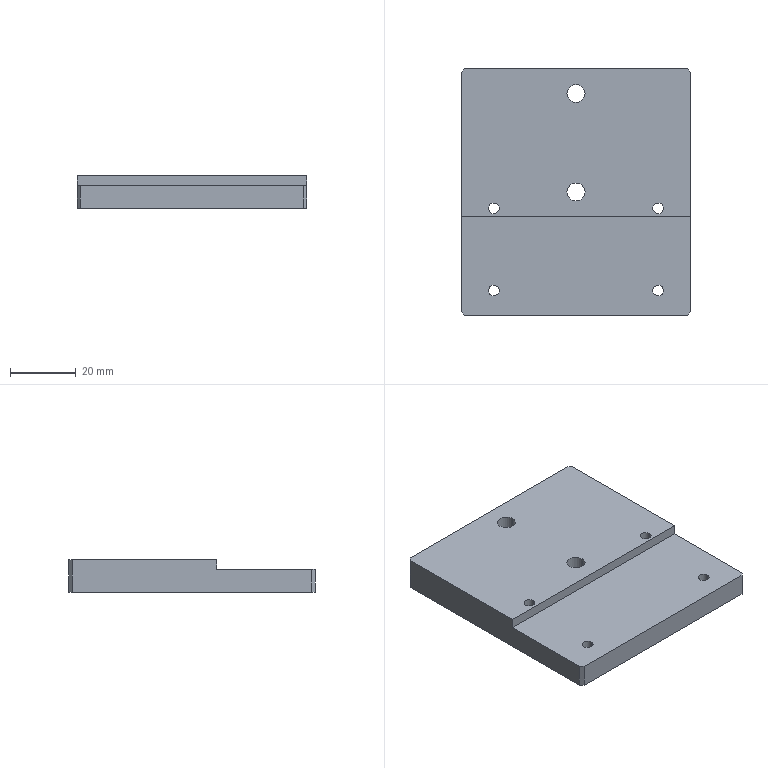Part | SolidWorks | features HoleWzd 2, Chamfer 1, Extrusion 1, ICE 1 | 1 solid | 30 faces | box 70 x 75 x 10 mm | volume 44793 mm3 | cylinder 16 | plane 14 | commonest cylinder face diameters 3.3 x8 5.5 x4 10 x4
STEP:
#1=CARTESIAN_POINT('',(40.,37.5,5.7));
#2=VERTEX_POINT('',#1);
#3=CARTESIAN_POINT('',(30.,37.5,5.7));
#4=VERTEX_POINT('',#3);
#5=CARTESIAN_POINT('',(35.,37.5,5.7));
#6=DIRECTION('',(0.,0.,-1.));
#7=DIRECTION('',(-1.,0.,0.));
#8=AXIS2_PLACEMENT_3D('',#5,#6,#7);
#9=CIRCLE('',#8,5.);
#10=EDGE_CURVE('',#2,#4,#9,.T.);
#11=ORIENTED_EDGE('',*,*,#10,.F.);
#12=CARTESIAN_POINT('',(40.,37.5,0.));
#13=VERTEX_POINT('',#12);
#14=CARTESIAN_POINT('',(40.,37.5,0.));
#15=DIRECTION('',(0.,0.,-1.));
#16=VECTOR('',#15,1000.);
#17=LINE('',#14,#16);
#18=EDGE_CURVE('',#2,#13,#17,.T.);
#19=ORIENTED_EDGE('',*,*,#18,.T.);
#20=CARTESIAN_POINT('',(30.,37.5,0.));
#21=VERTEX_POINT('',#20);
#22=CARTESIAN_POINT('',(35.,37.5,0.));
#23=DIRECTION('',(0.,0.,-1.));
#24=DIRECTION('',(-1.,0.,0.));
#25=AXIS2_PLACEMENT_3D('',#22,#23,#24);
#26=CIRCLE('',#25,5.);
#27=EDGE_CURVE('',#13,#21,#26,.T.);
#28=ORIENTED_EDGE('',*,*,#27,.T.);
#29=CARTESIAN_POINT('',(30.,37.5,0.));
#30=DIRECTION('',(0.,0.,-1.));
#31=VECTOR('',#30,1000.);
#32=LINE('',#29,#31);
#33=EDGE_CURVE('',#4,#21,#32,.T.);
#34=ORIENTED_EDGE('',*,*,#33,.F.);
#35=EDGE_LOOP('',(#11,#19,#28,#34));
#36=FACE_OUTER_BOUND('',#35,.T.);
#37=CARTESIAN_POINT('',(35.,37.5,0.));
#38=DIRECTION('',(0.,0.,-1.));
#39=DIRECTION('',(-1.,0.,0.));
#40=AXIS2_PLACEMENT_3D('',#37,#38,#39);
#41=CYLINDRICAL_SURFACE('',#40,5.);
#42=ADVANCED_FACE('',(#36),#41,.F.);
#43=CARTESIAN_POINT('',(37.75,37.5,10.));
#44=VERTEX_POINT('',#43);
#45=CARTESIAN_POINT('',(32.25,37.5,10.));
#46=VERTEX_POINT('',#45);
#47=CARTESIAN_POINT('',(35.,37.5,10.));
#48=DIRECTION('',(0.,0.,-1.));
#49=DIRECTION('',(-1.,0.,0.));
#50=AXIS2_PLACEMENT_3D('',#47,#48,#49);
#51=CIRCLE('',#50,2.75);
#52=EDGE_CURVE('',#44,#46,#51,.T.);
#53=ORIENTED_EDGE('',*,*,#52,.F.);
#54=CARTESIAN_POINT('',(37.75,37.5,5.7));
#55=VERTEX_POINT('',#54);
#56=CARTESIAN_POINT('',(37.75,37.5,0.));
#57=DIRECTION('',(0.,0.,-1.));
#58=VECTOR('',#57,1000.);
#59=LINE('',#56,#58);
#60=EDGE_CURVE('',#44,#55,#59,.T.);
#61=ORIENTED_EDGE('',*,*,#60,.T.);
#62=CARTESIAN_POINT('',(32.25,37.5,5.7));
#63=VERTEX_POINT('',#62);
#64=CARTESIAN_POINT('',(35.,37.5,5.7));
#65=DIRECTION('',(0.,0.,-1.));
#66=DIRECTION('',(-1.,0.,0.));
#67=AXIS2_PLACEMENT_3D('',#64,#65,#66);
#68=CIRCLE('',#67,2.75);
#69=EDGE_CURVE('',#55,#63,#68,.T.);
#70=ORIENTED_EDGE('',*,*,#69,.T.);
#71=CARTESIAN_POINT('',(32.25,37.5,0.));
#72=DIRECTION('',(0.,0.,-1.));
#73=VECTOR('',#72,1000.);
#74=LINE('',#71,#73);
#75=EDGE_CURVE('',#46,#63,#74,.T.);
#76=ORIENTED_EDGE('',*,*,#75,.F.);
#77=EDGE_LOOP('',(#53,#61,#70,#76));
#78=FACE_OUTER_BOUND('',#77,.T.);
#79=CARTESIAN_POINT('',(35.,37.5,0.));
#80=DIRECTION('',(0.,0.,-1.));
#81=DIRECTION('',(-1.,0.,0.));
#82=AXIS2_PLACEMENT_3D('',#79,#80,#81);
#83=CYLINDRICAL_SURFACE('',#82,2.75);
#84=ADVANCED_FACE('',(#78),#83,.F.);
#85=CARTESIAN_POINT('',(40.,67.5,5.7));
#86=VERTEX_POINT('',#85);
#87=CARTESIAN_POINT('',(30.,67.5,5.7));
#88=VERTEX_POINT('',#87);
#89=CARTESIAN_POINT('',(35.,67.5,5.7));
#90=DIRECTION('',(0.,0.,-1.));
#91=DIRECTION('',(-1.,0.,0.));
#92=AXIS2_PLACEMENT_3D('',#89,#90,#91);
#93=CIRCLE('',#92,5.);
#94=EDGE_CURVE('',#86,#88,#93,.T.);
#95=ORIENTED_EDGE('',*,*,#94,.F.);
#96=CARTESIAN_POINT('',(40.,67.5,0.));
#97=VERTEX_POINT('',#96);
#98=CARTESIAN_POINT('',(40.,67.5,0.));
#99=DIRECTION('',(0.,0.,-1.));
#100=VECTOR('',#99,1000.);
#101=LINE('',#98,#100);
#102=EDGE_CURVE('',#86,#97,#101,.T.);
#103=ORIENTED_EDGE('',*,*,#102,.T.);
#104=CARTESIAN_POINT('',(30.,67.5,0.));
#105=VERTEX_POINT('',#104);
#106=CARTESIAN_POINT('',(35.,67.5,0.));
#107=DIRECTION('',(0.,0.,-1.));
#108=DIRECTION('',(-1.,0.,0.));
#109=AXIS2_PLACEMENT_3D('',#106,#107,#108);
#110=CIRCLE('',#109,5.);
#111=EDGE_CURVE('',#97,#105,#110,.T.);
#112=ORIENTED_EDGE('',*,*,#111,.T.);
#113=CARTESIAN_POINT('',(30.,67.5,0.));
#114=DIRECTION('',(0.,0.,-1.));
#115=VECTOR('',#114,1000.);
#116=LINE('',#113,#115);
#117=EDGE_CURVE('',#88,#105,#116,.T.);
#118=ORIENTED_EDGE('',*,*,#117,.F.);
#119=EDGE_LOOP('',(#95,#103,#112,#118));
#120=FACE_OUTER_BOUND('',#119,.T.);
#121=CARTESIAN_POINT('',(35.,67.5,0.));
#122=DIRECTION('',(0.,0.,-1.));
#123=DIRECTION('',(-1.,0.,0.));
#124=AXIS2_PLACEMENT_3D('',#121,#122,#123);
#125=CYLINDRICAL_SURFACE('',#124,5.);
#126=ADVANCED_FACE('',(#120),#125,.F.);
#127=CARTESIAN_POINT('',(37.75,67.5,10.));
#128=VERTEX_POINT('',#127);
#129=CARTESIAN_POINT('',(32.25,67.5,10.));
#130=VERTEX_POINT('',#129);
#131=CARTESIAN_POINT('',(35.,67.5,10.));
#132=DIRECTION('',(0.,0.,-1.));
#133=DIRECTION('',(-1.,0.,0.));
#134=AXIS2_PLACEMENT_3D('',#131,#132,#133);
#135=CIRCLE('',#134,2.75);
#136=EDGE_CURVE('',#128,#130,#135,.T.);
#137=ORIENTED_EDGE('',*,*,#136,.F.);
#138=CARTESIAN_POINT('',(37.75,67.5,5.7));
#139=VERTEX_POINT('',#138);
#140=CARTESIAN_POINT('',(37.75,67.5,0.));
#141=DIRECTION('',(0.,0.,-1.));
#142=VECTOR('',#141,1000.);
#143=LINE('',#140,#142);
#144=EDGE_CURVE('',#128,#139,#143,.T.);
#145=ORIENTED_EDGE('',*,*,#144,.T.);
#146=CARTESIAN_POINT('',(32.25,67.5,5.7));
#147=VERTEX_POINT('',#146);
#148=CARTESIAN_POINT('',(35.,67.5,5.7));
#149=DIRECTION('',(0.,0.,-1.));
#150=DIRECTION('',(-1.,0.,0.));
#151=AXIS2_PLACEMENT_3D('',#148,#149,#150);
#152=CIRCLE('',#151,2.75);
#153=EDGE_CURVE('',#139,#147,#152,.T.);
#154=ORIENTED_EDGE('',*,*,#153,.T.);
#155=CARTESIAN_POINT('',(32.25,67.5,0.));
#156=DIRECTION('',(0.,0.,-1.));
#157=VECTOR('',#156,1000.);
#158=LINE('',#155,#157);
#159=EDGE_CURVE('',#130,#147,#158,.T.);
#160=ORIENTED_EDGE('',*,*,#159,.F.);
#161=EDGE_LOOP('',(#137,#145,#154,#160));
#162=FACE_OUTER_BOUND('',#161,.T.);
#163=CARTESIAN_POINT('',(35.,67.5,0.));
#164=DIRECTION('',(0.,0.,-1.));
#165=DIRECTION('',(-1.,0.,0.));
#166=AXIS2_PLACEMENT_3D('',#163,#164,#165);
#167=CYLINDRICAL_SURFACE('',#166,2.75);
#168=ADVANCED_FACE('',(#162),#167,.F.);
#169=CARTESIAN_POINT('',(11.65,7.5,7.));
#170=VERTEX_POINT('',#169);
#171=CARTESIAN_POINT('',(8.35,7.5,7.));
#172=VERTEX_POINT('',#171);
#173=CARTESIAN_POINT('',(10.,7.5,7.));
#174=DIRECTION('',(0.,0.,-1.));
#175=DIRECTION('',(-1.,0.,0.));
#176=AXIS2_PLACEMENT_3D('',#173,#174,#175);
#177=CIRCLE('',#176,1.65);
#178=EDGE_CURVE('',#170,#172,#177,.T.);
#179=ORIENTED_EDGE('',*,*,#178,.F.);
#180=CARTESIAN_POINT('',(11.65,7.5,0.));
#181=VERTEX_POINT('',#180);
#182=CARTESIAN_POINT('',(11.65,7.5,0.));
#183=DIRECTION('',(0.,0.,-1.));
#184=VECTOR('',#183,1000.);
#185=LINE('',#182,#184);
#186=EDGE_CURVE('',#170,#181,#185,.T.);
#187=ORIENTED_EDGE('',*,*,#186,.T.);
#188=CARTESIAN_POINT('',(8.35,7.5,0.));
#189=VERTEX_POINT('',#188);
#190=CARTESIAN_POINT('',(10.,7.5,0.));
#191=DIRECTION('',(0.,0.,-1.));
#192=DIRECTION('',(-1.,0.,0.));
#193=AXIS2_PLACEMENT_3D('',#190,#191,#192);
#194=CIRCLE('',#193,1.65);
#195=EDGE_CURVE('',#181,#189,#194,.T.);
#196=ORIENTED_EDGE('',*,*,#195,.T.);
#197=CARTESIAN_POINT('',(8.35,7.5,0.));
#198=DIRECTION('',(0.,0.,-1.));
#199=VECTOR('',#198,1000.);
#200=LINE('',#197,#199);
#201=EDGE_CURVE('',#172,#189,#200,.T.);
#202=ORIENTED_EDGE('',*,*,#201,.F.);
#203=EDGE_LOOP('',(#179,#187,#196,#202));
#204=FACE_OUTER_BOUND('',#203,.T.);
#205=CARTESIAN_POINT('',(10.,7.5,0.));
#206=DIRECTION('',(0.,0.,-1.));
#207=DIRECTION('',(-1.,0.,0.));
#208=AXIS2_PLACEMENT_3D('',#205,#206,#207);
#209=CYLINDRICAL_SURFACE('',#208,1.65);
#210=ADVANCED_FACE('',(#204),#209,.F.);
#211=CARTESIAN_POINT('',(11.65,32.5,10.));
#212=VERTEX_POINT('',#211);
#213=CARTESIAN_POINT('',(8.35,32.5,10.));
#214=VERTEX_POINT('',#213);
#215=CARTESIAN_POINT('',(10.,32.5,10.));
#216=DIRECTION('',(0.,0.,-1.));
#217=DIRECTION('',(-1.,0.,0.));
#218=AXIS2_PLACEMENT_3D('',#215,#216,#217);
#219=CIRCLE('',#218,1.65);
#220=EDGE_CURVE('',#212,#214,#219,.T.);
#221=ORIENTED_EDGE('',*,*,#220,.F.);
#222=CARTESIAN_POINT('',(11.65,32.5,0.));
#223=VERTEX_POINT('',#222);
#224=CARTESIAN_POINT('',(11.65,32.5,0.));
#225=DIRECTION('',(0.,0.,-1.));
#226=VECTOR('',#225,1000.);
#227=LINE('',#224,#226);
#228=EDGE_CURVE('',#212,#223,#227,.T.);
#229=ORIENTED_EDGE('',*,*,#228,.T.);
#230=CARTESIAN_POINT('',(8.35,32.5,0.));
#231=VERTEX_POINT('',#230);
#232=CARTESIAN_POINT('',(10.,32.5,0.));
#233=DIRECTION('',(0.,0.,-1.));
#234=DIRECTION('',(-1.,0.,0.));
#235=AXIS2_PLACEMENT_3D('',#232,#233,#234);
#236=CIRCLE('',#235,1.65);
#237=EDGE_CURVE('',#223,#231,#236,.T.);
#238=ORIENTED_EDGE('',*,*,#237,.T.);
#239=CARTESIAN_POINT('',(8.35,32.5,0.));
#240=DIRECTION('',(0.,0.,-1.));
#241=VECTOR('',#240,1000.);
#242=LINE('',#239,#241);
#243=EDGE_CURVE('',#214,#231,#242,.T.);
#244=ORIENTED_EDGE('',*,*,#243,.F.);
#245=EDGE_LOOP('',(#221,#229,#238,#244));
#246=FACE_OUTER_BOUND('',#245,.T.);
#247=CARTESIAN_POINT('',(10.,32.5,0.));
#248=DIRECTION('',(0.,0.,-1.));
#249=DIRECTION('',(-1.,0.,0.));
#250=AXIS2_PLACEMENT_3D('',#247,#248,#249);
#251=CYLINDRICAL_SURFACE('',#250,1.65);
#252=ADVANCED_FACE('',(#246),#251,.F.);
#253=CARTESIAN_POINT('',(61.65,7.5,7.));
#254=VERTEX_POINT('',#253);
#255=CARTESIAN_POINT('',(58.35,7.5,7.));
#256=VERTEX_POINT('',#255);
#257=CARTESIAN_POINT('',(60.,7.5,7.));
#258=DIRECTION('',(0.,0.,-1.));
#259=DIRECTION('',(-1.,0.,0.));
#260=AXIS2_PLACEMENT_3D('',#257,#258,#259);
#261=CIRCLE('',#260,1.65);
#262=EDGE_CURVE('',#254,#256,#261,.T.);
#263=ORIENTED_EDGE('',*,*,#262,.F.);
#264=CARTESIAN_POINT('',(61.65,7.5,0.));
#265=VERTEX_POINT('',#264);
#266=CARTESIAN_POINT('',(61.65,7.5,0.));
#267=DIRECTION('',(0.,0.,-1.));
#268=VECTOR('',#267,1000.);
#269=LINE('',#266,#268);
#270=EDGE_CURVE('',#254,#265,#269,.T.);
#271=ORIENTED_EDGE('',*,*,#270,.T.);
#272=CARTESIAN_POINT('',(58.35,7.5,0.));
#273=VERTEX_POINT('',#272);
#274=CARTESIAN_POINT('',(60.,7.5,0.));
#275=DIRECTION('',(0.,0.,-1.));
#276=DIRECTION('',(-1.,0.,0.));
#277=AXIS2_PLACEMENT_3D('',#274,#275,#276);
#278=CIRCLE('',#277,1.65);
#279=EDGE_CURVE('',#265,#273,#278,.T.);
#280=ORIENTED_EDGE('',*,*,#279,.T.);
#281=CARTESIAN_POINT('',(58.35,7.5,0.));
#282=DIRECTION('',(0.,0.,-1.));
#283=VECTOR('',#282,1000.);
#284=LINE('',#281,#283);
#285=EDGE_CURVE('',#256,#273,#284,.T.);
#286=ORIENTED_EDGE('',*,*,#285,.F.);
#287=EDGE_LOOP('',(#263,#271,#280,#286));
#288=FACE_OUTER_BOUND('',#287,.T.);
#289=CARTESIAN_POINT('',(60.,7.5,0.));
#290=DIRECTION('',(0.,0.,-1.));
#291=DIRECTION('',(-1.,0.,0.));
#292=AXIS2_PLACEMENT_3D('',#289,#290,#291);
#293=CYLINDRICAL_SURFACE('',#292,1.65);
#294=ADVANCED_FACE('',(#288),#293,.F.);
#295=CARTESIAN_POINT('',(61.65,32.5,10.));
#296=VERTEX_POINT('',#295);
#297=CARTESIAN_POINT('',(58.35,32.5,10.));
#298=VERTEX_POINT('',#297);
#299=CARTESIAN_POINT('',(60.,32.5,10.));
#300=DIRECTION('',(0.,0.,-1.));
#301=DIRECTION('',(-1.,0.,0.));
#302=AXIS2_PLACEMENT_3D('',#299,#300,#301);
#303=CIRCLE('',#302,1.65);
#304=EDGE_CURVE('',#296,#298,#303,.T.);
#305=ORIENTED_EDGE('',*,*,#304,.F.);
#306=CARTESIAN_POINT('',(61.65,32.5,0.));
#307=VERTEX_POINT('',#306);
#308=CARTESIAN_POINT('',(61.65,32.5,0.));
#309=DIRECTION('',(0.,0.,-1.));
#310=VECTOR('',#309,1000.);
#311=LINE('',#308,#310);
#312=EDGE_CURVE('',#296,#307,#311,.T.);
#313=ORIENTED_EDGE('',*,*,#312,.T.);
#314=CARTESIAN_POINT('',(58.35,32.5,0.));
#315=VERTEX_POINT('',#314);
#316=CARTESIAN_POINT('',(60.,32.5,0.));
#317=DIRECTION('',(0.,0.,-1.));
#318=DIRECTION('',(-1.,0.,0.));
#319=AXIS2_PLACEMENT_3D('',#316,#317,#318);
#320=CIRCLE('',#319,1.65);
#321=EDGE_CURVE('',#307,#315,#320,.T.);
#322=ORIENTED_EDGE('',*,*,#321,.T.);
#323=CARTESIAN_POINT('',(58.35,32.5,0.));
#324=DIRECTION('',(0.,0.,-1.));
#325=VECTOR('',#324,1000.);
#326=LINE('',#323,#325);
#327=EDGE_CURVE('',#298,#315,#326,.T.);
#328=ORIENTED_EDGE('',*,*,#327,.F.);
#329=EDGE_LOOP('',(#305,#313,#322,#328));
#330=FACE_OUTER_BOUND('',#329,.T.);
#331=CARTESIAN_POINT('',(60.,32.5,0.));
#332=DIRECTION('',(0.,0.,-1.));
#333=DIRECTION('',(-1.,0.,0.));
#334=AXIS2_PLACEMENT_3D('',#331,#332,#333);
#335=CYLINDRICAL_SURFACE('',#334,1.65);
#336=ADVANCED_FACE('',(#330),#335,.F.);
#337=CARTESIAN_POINT('',(0.,74.,0.));
#338=VERTEX_POINT('',#337);
#339=CARTESIAN_POINT('',(0.,1.,0.));
#340=VERTEX_POINT('',#339);
#341=CARTESIAN_POINT('',(0.,0.,0.));
#342=DIRECTION('',(0.,-1.,0.));
#343=VECTOR('',#342,1000.);
#344=LINE('',#341,#343);
#345=EDGE_CURVE('',#338,#340,#344,.T.);
#346=ORIENTED_EDGE('',*,*,#345,.T.);
#347=CARTESIAN_POINT('',(0.,1.,7.));
#348=VERTEX_POINT('',#347);
#349=CARTESIAN_POINT('',(0.,1.,10.));
#350=DIRECTION('',(0.,0.,1.));
#351=VECTOR('',#350,1000.);
#352=LINE('',#349,#351);
#353=EDGE_CURVE('',#340,#348,#352,.T.);
#354=ORIENTED_EDGE('',*,*,#353,.T.);
#355=CARTESIAN_POINT('',(0.,30.,7.));
#356=VERTEX_POINT('',#355);
#357=CARTESIAN_POINT('',(0.,0.,7.));
#358=DIRECTION('',(0.,-1.,0.));
#359=VECTOR('',#358,1000.);
#360=LINE('',#357,#359);
#361=EDGE_CURVE('',#356,#348,#360,.T.);
#362=ORIENTED_EDGE('',*,*,#361,.F.);
#363=CARTESIAN_POINT('',(0.,30.,10.));
#364=VERTEX_POINT('',#363);
#365=CARTESIAN_POINT('',(0.,30.,10.));
#366=DIRECTION('',(0.,0.,-1.));
#367=VECTOR('',#366,1000.);
#368=LINE('',#365,#367);
#369=EDGE_CURVE('',#364,#356,#368,.T.);
#370=ORIENTED_EDGE('',*,*,#369,.F.);
#371=CARTESIAN_POINT('',(0.,74.,10.));
#372=VERTEX_POINT('',#371);
#373=CARTESIAN_POINT('',(0.,0.,10.));
#374=DIRECTION('',(0.,-1.,0.));
#375=VECTOR('',#374,1000.);
#376=LINE('',#373,#375);
#377=EDGE_CURVE('',#372,#364,#376,.T.);
#378=ORIENTED_EDGE('',*,*,#377,.F.);
#379=CARTESIAN_POINT('',(0.,74.,10.));
#380=DIRECTION('',(0.,0.,-1.));
#381=VECTOR('',#380,1000.);
#382=LINE('',#379,#381);
#383=EDGE_CURVE('',#372,#338,#382,.T.);
#384=ORIENTED_EDGE('',*,*,#383,.T.);
#385=EDGE_LOOP('',(#346,#354,#362,#370,#378,#384));
#386=FACE_OUTER_BOUND('',#385,.T.);
#387=CARTESIAN_POINT('',(0.,0.,10.));
#388=DIRECTION('',(1.,0.,0.));
#389=DIRECTION('',(0.,0.,-1.));
#390=AXIS2_PLACEMENT_3D('',#387,#388,#389);
#391=PLANE('',#390);
#392=ADVANCED_FACE('',(#386),#391,.F.);
#393=CARTESIAN_POINT('',(1.,0.,0.));
#394=VERTEX_POINT('',#393);
#395=CARTESIAN_POINT('',(69.,0.,0.));
#396=VERTEX_POINT('',#395);
#397=CARTESIAN_POINT('',(0.,0.,0.));
#398=DIRECTION('',(1.,0.,0.));
#399=VECTOR('',#398,1000.);
#400=LINE('',#397,#399);
#401=EDGE_CURVE('',#394,#396,#400,.T.);
#402=ORIENTED_EDGE('',*,*,#401,.T.);
#403=CARTESIAN_POINT('',(69.,0.,7.));
#404=VERTEX_POINT('',#403);
#405=CARTESIAN_POINT('',(69.,0.,10.));
#406=DIRECTION('',(0.,0.,1.));
#407=VECTOR('',#406,1000.);
#408=LINE('',#405,#407);
#409=EDGE_CURVE('',#396,#404,#408,.T.);
#410=ORIENTED_EDGE('',*,*,#409,.T.);
#411=CARTESIAN_POINT('',(1.,0.,7.));
#412=VERTEX_POINT('',#411);
#413=CARTESIAN_POINT('',(70.,0.,7.));
#414=DIRECTION('',(-1.,0.,0.));
#415=VECTOR('',#414,1000.);
#416=LINE('',#413,#415);
#417=EDGE_CURVE('',#404,#412,#416,.T.);
#418=ORIENTED_EDGE('',*,*,#417,.T.);
#419=CARTESIAN_POINT('',(1.,0.,10.));
#420=DIRECTION('',(0.,0.,-1.));
#421=VECTOR('',#420,1000.);
#422=LINE('',#419,#421);
#423=EDGE_CURVE('',#412,#394,#422,.T.);
#424=ORIENTED_EDGE('',*,*,#423,.T.);
#425=EDGE_LOOP('',(#402,#410,#418,#424));
#426=FACE_OUTER_BOUND('',#425,.T.);
#427=CARTESIAN_POINT('',(0.,0.,10.));
#428=DIRECTION('',(0.,1.,0.));
#429=DIRECTION('',(0.,0.,1.));
#430=AXIS2_PLACEMENT_3D('',#427,#428,#429);
#431=PLANE('',#430);
#432=ADVANCED_FACE('',(#426),#431,.F.);
#433=CARTESIAN_POINT('',(70.,30.,7.));
#434=VERTEX_POINT('',#433);
#435=CARTESIAN_POINT('',(70.,1.,7.));
#436=VERTEX_POINT('',#435);
#437=CARTESIAN_POINT('',(70.,0.,7.));
#438=DIRECTION('',(0.,-1.,0.));
#439=VECTOR('',#438,1000.);
#440=LINE('',#437,#439);
#441=EDGE_CURVE('',#434,#436,#440,.T.);
#442=ORIENTED_EDGE('',*,*,#441,.T.);
#443=CARTESIAN_POINT('',(70.,1.,0.));
#444=VERTEX_POINT('',#443);
#445=CARTESIAN_POINT('',(70.,1.,10.));
#446=DIRECTION('',(0.,0.,-1.));
#447=VECTOR('',#446,1000.);
#448=LINE('',#445,#447);
#449=EDGE_CURVE('',#436,#444,#448,.T.);
#450=ORIENTED_EDGE('',*,*,#449,.T.);
#451=CARTESIAN_POINT('',(70.,74.,0.));
#452=VERTEX_POINT('',#451);
#453=CARTESIAN_POINT('',(70.,0.,0.));
#454=DIRECTION('',(0.,1.,0.));
#455=VECTOR('',#454,1000.);
#456=LINE('',#453,#455);
#457=EDGE_CURVE('',#444,#452,#456,.T.);
#458=ORIENTED_EDGE('',*,*,#457,.T.);
#459=CARTESIAN_POINT('',(70.,74.,10.));
#460=VERTEX_POINT('',#459);
#461=CARTESIAN_POINT('',(70.,74.,10.));
#462=DIRECTION('',(0.,0.,1.));
#463=VECTOR('',#462,1000.);
#464=LINE('',#461,#463);
#465=EDGE_CURVE('',#452,#460,#464,.T.);
#466=ORIENTED_EDGE('',*,*,#465,.T.);
#467=CARTESIAN_POINT('',(70.,30.,10.));
#468=VERTEX_POINT('',#467);
#469=CARTESIAN_POINT('',(70.,0.,10.));
#470=DIRECTION('',(0.,1.,0.));
#471=VECTOR('',#470,1000.);
#472=LINE('',#469,#471);
#473=EDGE_CURVE('',#468,#460,#472,.T.);
#474=ORIENTED_EDGE('',*,*,#473,.F.);
#475=CARTESIAN_POINT('',(70.,30.,10.));
#476=DIRECTION('',(0.,0.,-1.));
#477=VECTOR('',#476,1000.);
#478=LINE('',#475,#477);
#479=EDGE_CURVE('',#468,#434,#478,.T.);
#480=ORIENTED_EDGE('',*,*,#479,.T.);
#481=EDGE_LOOP('',(#442,#450,#458,#466,#474,#480));
#482=FACE_OUTER_BOUND('',#481,.T.);
#483=CARTESIAN_POINT('',(70.,0.,10.));
#484=DIRECTION('',(-1.,0.,0.));
#485=DIRECTION('',(0.,0.,1.));
#486=AXIS2_PLACEMENT_3D('',#483,#484,#485);
#487=PLANE('',#486);
#488=ADVANCED_FACE('',(#482),#487,.F.);
#489=CARTESIAN_POINT('',(69.,75.,0.));
#490=VERTEX_POINT('',#489);
#491=CARTESIAN_POINT('',(1.,75.,0.));
#492=VERTEX_POINT('',#491);
#493=CARTESIAN_POINT('',(0.,75.,0.));
#494=DIRECTION('',(-1.,0.,0.));
#495=VECTOR('',#494,1000.);
#496=LINE('',#493,#495);
#497=EDGE_CURVE('',#490,#492,#496,.T.);
#498=ORIENTED_EDGE('',*,*,#497,.T.);
#499=CARTESIAN_POINT('',(1.,75.,10.));
#500=VERTEX_POINT('',#499);
#501=CARTESIAN_POINT('',(1.,75.,10.));
#502=DIRECTION('',(0.,0.,1.));
#503=VECTOR('',#502,1000.);
#504=LINE('',#501,#503);
#505=EDGE_CURVE('',#492,#500,#504,.T.);
#506=ORIENTED_EDGE('',*,*,#505,.T.);
#507=CARTESIAN_POINT('',(69.,75.,10.));
#508=VERTEX_POINT('',#507);
#509=CARTESIAN_POINT('',(0.,75.,10.));
#510=DIRECTION('',(-1.,0.,0.));
#511=VECTOR('',#510,1000.);
#512=LINE('',#509,#511);
#513=EDGE_CURVE('',#508,#500,#512,.T.);
#514=ORIENTED_EDGE('',*,*,#513,.F.);
#515=CARTESIAN_POINT('',(69.,75.,10.));
#516=DIRECTION('',(0.,0.,-1.));
#517=VECTOR('',#516,1000.);
#518=LINE('',#515,#517);
#519=EDGE_CURVE('',#508,#490,#518,.T.);
#520=ORIENTED_EDGE('',*,*,#519,.T.);
#521=EDGE_LOOP('',(#498,#506,#514,#520));
#522=FACE_OUTER_BOUND('',#521,.T.);
#523=CARTESIAN_POINT('',(0.,75.,10.));
#524=DIRECTION('',(0.,-1.,0.));
#525=DIRECTION('',(0.,0.,-1.));
#526=AXIS2_PLACEMENT_3D('',#523,#524,#525);
#527=PLANE('',#526);
#528=ADVANCED_FACE('',(#522),#527,.F.);
#529=CARTESIAN_POINT('',(35.,37.5,10.));
#530=DIRECTION('',(0.,0.,-1.));
#531=DIRECTION('',(-1.,0.,0.));
#532=AXIS2_PLACEMENT_3D('',#529,#530,#531);
#533=CIRCLE('',#532,2.75);
#534=EDGE_CURVE('',#46,#44,#533,.T.);
#535=ORIENTED_EDGE('',*,*,#534,.T.);
#536=ORIENTED_EDGE('',*,*,#52,.T.);
#537=EDGE_LOOP('',(#535,#536));
#538=FACE_BOUND('',#537,.T.);
#539=CARTESIAN_POINT('',(35.,67.5,10.));
#540=DIRECTION('',(0.,0.,-1.));
#541=DIRECTION('',(-1.,0.,0.));
#542=AXIS2_PLACEMENT_3D('',#539,#540,#541);
#543=CIRCLE('',#542,2.75);
#544=EDGE_CURVE('',#130,#128,#543,.T.);
#545=ORIENTED_EDGE('',*,*,#544,.T.);
#546=ORIENTED_EDGE('',*,*,#136,.T.);
#547=EDGE_LOOP('',(#545,#546));
#548=FACE_BOUND('',#547,.T.);
#549=CARTESIAN_POINT('',(10.,32.5,10.));
#550=DIRECTION('',(0.,0.,-1.));
#551=DIRECTION('',(-1.,0.,0.));
#552=AXIS2_PLACEMENT_3D('',#549,#550,#551);
#553=CIRCLE('',#552,1.65);
#554=EDGE_CURVE('',#214,#212,#553,.T.);
#555=ORIENTED_EDGE('',*,*,#554,.T.);
#556=ORIENTED_EDGE('',*,*,#220,.T.);
#557=EDGE_LOOP('',(#555,#556));
#558=FACE_BOUND('',#557,.T.);
#559=CARTESIAN_POINT('',(60.,32.5,10.));
#560=DIRECTION('',(0.,0.,-1.));
#561=DIRECTION('',(-1.,0.,0.));
#562=AXIS2_PLACEMENT_3D('',#559,#560,#561);
#563=CIRCLE('',#562,1.65);
#564=EDGE_CURVE('',#298,#296,#563,.T.);
#565=ORIENTED_EDGE('',*,*,#564,.T.);
#566=ORIENTED_EDGE('',*,*,#304,.T.);
#567=EDGE_LOOP('',(#565,#566));
#568=FACE_BOUND('',#567,.T.);
#569=ORIENTED_EDGE('',*,*,#513,.T.);
#570=CARTESIAN_POINT('',(0.,74.,10.));
#571=DIRECTION('',(-0.7071,-0.7071,0.));
#572=VECTOR('',#571,1000.);
#573=LINE('',#570,#572);
#574=EDGE_CURVE('',#500,#372,#573,.T.);
#575=ORIENTED_EDGE('',*,*,#574,.T.);
#576=ORIENTED_EDGE('',*,*,#377,.T.);
#577=CARTESIAN_POINT('',(70.,30.,10.));
#578=DIRECTION('',(-1.,0.,0.));
#579=VECTOR('',#578,1000.);
#580=LINE('',#577,#579);
#581=EDGE_CURVE('',#468,#364,#580,.T.);
#582=ORIENTED_EDGE('',*,*,#581,.F.);
#583=ORIENTED_EDGE('',*,*,#473,.T.);
#584=CARTESIAN_POINT('',(69.,75.,10.));
#585=DIRECTION('',(-0.7071,0.7071,0.));
#586=VECTOR('',#585,1000.);
#587=LINE('',#584,#586);
#588=EDGE_CURVE('',#460,#508,#587,.T.);
#589=ORIENTED_EDGE('',*,*,#588,.T.);
#590=EDGE_LOOP('',(#569,#575,#576,#582,#583,#589));
#591=FACE_OUTER_BOUND('',#590,.T.);
#592=CARTESIAN_POINT('',(0.,75.,10.));
#593=DIRECTION('',(0.,0.,-1.));
#594=DIRECTION('',(-1.,0.,0.));
#595=AXIS2_PLACEMENT_3D('',#592,#593,#594);
#596=PLANE('',#595);
#597=ADVANCED_FACE('',(#538,#548,#558,#568,#591),#596,.F.);
#598=CARTESIAN_POINT('',(35.,37.5,0.));
#599=DIRECTION('',(0.,0.,-1.));
#600=DIRECTION('',(-1.,0.,0.));
#601=AXIS2_PLACEMENT_3D('',#598,#599,#600);
#602=CIRCLE('',#601,5.);
#603=EDGE_CURVE('',#21,#13,#602,.T.);
#604=ORIENTED_EDGE('',*,*,#603,.F.);
#605=ORIENTED_EDGE('',*,*,#27,.F.);
#606=EDGE_LOOP('',(#604,#605));
#607=FACE_BOUND('',#606,.T.);
#608=CARTESIAN_POINT('',(35.,67.5,0.));
#609=DIRECTION('',(0.,0.,-1.));
#610=DIRECTION('',(-1.,0.,0.));
#611=AXIS2_PLACEMENT_3D('',#608,#609,#610);
#612=CIRCLE('',#611,5.);
#613=EDGE_CURVE('',#105,#97,#612,.T.);
#614=ORIENTED_EDGE('',*,*,#613,.F.);
#615=ORIENTED_EDGE('',*,*,#111,.F.);
#616=EDGE_LOOP('',(#614,#615));
#617=FACE_BOUND('',#616,.T.);
#618=CARTESIAN_POINT('',(10.,7.5,0.));
#619=DIRECTION('',(0.,0.,-1.));
#620=DIRECTION('',(-1.,0.,0.));
#621=AXIS2_PLACEMENT_3D('',#618,#619,#620);
#622=CIRCLE('',#621,1.65);
#623=EDGE_CURVE('',#189,#181,#622,.T.);
#624=ORIENTED_EDGE('',*,*,#623,.F.);
#625=ORIENTED_EDGE('',*,*,#195,.F.);
#626=EDGE_LOOP('',(#624,#625));
#627=FACE_BOUND('',#626,.T.);
#628=CARTESIAN_POINT('',(10.,32.5,0.));
#629=DIRECTION('',(0.,0.,-1.));
#630=DIRECTION('',(-1.,0.,0.));
#631=AXIS2_PLACEMENT_3D('',#628,#629,#630);
#632=CIRCLE('',#631,1.65);
#633=EDGE_CURVE('',#231,#223,#632,.T.);
#634=ORIENTED_EDGE('',*,*,#633,.F.);
#635=ORIENTED_EDGE('',*,*,#237,.F.);
#636=EDGE_LOOP('',(#634,#635));
#637=FACE_BOUND('',#636,.T.);
#638=CARTESIAN_POINT('',(60.,7.5,0.));
#639=DIRECTION('',(0.,0.,-1.));
#640=DIRECTION('',(-1.,0.,0.));
#641=AXIS2_PLACEMENT_3D('',#638,#639,#640);
#642=CIRCLE('',#641,1.65);
#643=EDGE_CURVE('',#273,#265,#642,.T.);
#644=ORIENTED_EDGE('',*,*,#643,.F.);
#645=ORIENTED_EDGE('',*,*,#279,.F.);
#646=EDGE_LOOP('',(#644,#645));
#647=FACE_BOUND('',#646,.T.);
#648=CARTESIAN_POINT('',(60.,32.5,0.));
#649=DIRECTION('',(0.,0.,-1.));
#650=DIRECTION('',(-1.,0.,0.));
#651=AXIS2_PLACEMENT_3D('',#648,#649,#650);
#652=CIRCLE('',#651,1.65);
#653=EDGE_CURVE('',#315,#307,#652,.T.);
#654=ORIENTED_EDGE('',*,*,#653,.F.);
#655=ORIENTED_EDGE('',*,*,#321,.F.);
#656=EDGE_LOOP('',(#654,#655));
#657=FACE_BOUND('',#656,.T.);
#658=ORIENTED_EDGE('',*,*,#457,.F.);
#659=CARTESIAN_POINT('',(72.,3.,0.));
#660=DIRECTION('',(-0.7071,-0.7071,0.));
#661=VECTOR('',#660,1000.);
#662=LINE('',#659,#661);
#663=EDGE_CURVE('',#444,#396,#662,.T.);
#664=ORIENTED_EDGE('',*,*,#663,.T.);
#665=ORIENTED_EDGE('',*,*,#401,.F.);
#666=CARTESIAN_POINT('',(-37.,38.,0.));
#667=DIRECTION('',(-0.7071,0.7071,0.));
#668=VECTOR('',#667,1000.);
#669=LINE('',#666,#668);
#670=EDGE_CURVE('',#394,#340,#669,.T.);
#671=ORIENTED_EDGE('',*,*,#670,.T.);
#672=ORIENTED_EDGE('',*,*,#345,.F.);
#673=CARTESIAN_POINT('',(0.5,74.5,0.));
#674=DIRECTION('',(0.7071,0.7071,0.));
#675=VECTOR('',#674,1000.);
#676=LINE('',#673,#675);
#677=EDGE_CURVE('',#338,#492,#676,.T.);
#678=ORIENTED_EDGE('',*,*,#677,.T.);
#679=ORIENTED_EDGE('',*,*,#497,.F.);
#680=CARTESIAN_POINT('',(34.5,109.5,0.));
#681=DIRECTION('',(0.7071,-0.7071,0.));
#682=VECTOR('',#681,1000.);
#683=LINE('',#680,#682);
#684=EDGE_CURVE('',#490,#452,#683,.T.);
#685=ORIENTED_EDGE('',*,*,#684,.T.);
#686=EDGE_LOOP('',(#658,#664,#665,#671,#672,#678,#679,#685));
#687=FACE_OUTER_BOUND('',#686,.T.);
#688=CARTESIAN_POINT('',(0.,75.,0.));
#689=DIRECTION('',(0.,0.,-1.));
#690=DIRECTION('',(-1.,0.,0.));
#691=AXIS2_PLACEMENT_3D('',#688,#689,#690);
#692=PLANE('',#691);
#693=ADVANCED_FACE('',(#607,#617,#627,#637,#647,#657,#687),#692,.T.);
#694=CARTESIAN_POINT('',(10.,7.5,7.));
#695=DIRECTION('',(0.,0.,-1.));
#696=DIRECTION('',(-1.,0.,0.));
#697=AXIS2_PLACEMENT_3D('',#694,#695,#696);
#698=CIRCLE('',#697,1.65);
#699=EDGE_CURVE('',#172,#170,#698,.T.);
#700=ORIENTED_EDGE('',*,*,#699,.T.);
#701=ORIENTED_EDGE('',*,*,#178,.T.);
#702=EDGE_LOOP('',(#700,#701));
#703=FACE_BOUND('',#702,.T.);
#704=CARTESIAN_POINT('',(60.,7.5,7.));
#705=DIRECTION('',(0.,0.,-1.));
#706=DIRECTION('',(-1.,0.,0.));
#707=AXIS2_PLACEMENT_3D('',#704,#705,#706);
#708=CIRCLE('',#707,1.65);
#709=EDGE_CURVE('',#256,#254,#708,.T.);
#710=ORIENTED_EDGE('',*,*,#709,.T.);
#711=ORIENTED_EDGE('',*,*,#262,.T.);
#712=EDGE_LOOP('',(#710,#711));
#713=FACE_BOUND('',#712,.T.);
#714=ORIENTED_EDGE('',*,*,#417,.F.);
#715=CARTESIAN_POINT('',(70.,1.,7.));
#716=DIRECTION('',(0.7071,0.7071,0.));
#717=VECTOR('',#716,1000.);
#718=LINE('',#715,#717);
#719=EDGE_CURVE('',#404,#436,#718,.T.);
#720=ORIENTED_EDGE('',*,*,#719,.T.);
#721=ORIENTED_EDGE('',*,*,#441,.F.);
#722=CARTESIAN_POINT('',(70.,30.,7.));
#723=DIRECTION('',(-1.,0.,0.));
#724=VECTOR('',#723,1000.);
#725=LINE('',#722,#724);
#726=EDGE_CURVE('',#434,#356,#725,.T.);
#727=ORIENTED_EDGE('',*,*,#726,.T.);
#728=ORIENTED_EDGE('',*,*,#361,.T.);
#729=CARTESIAN_POINT('',(1.,0.,7.));
#730=DIRECTION('',(0.7071,-0.7071,0.));
#731=VECTOR('',#730,1000.);
#732=LINE('',#729,#731);
#733=EDGE_CURVE('',#348,#412,#732,.T.);
#734=ORIENTED_EDGE('',*,*,#733,.T.);
#735=EDGE_LOOP('',(#714,#720,#721,#727,#728,#734));
#736=FACE_OUTER_BOUND('',#735,.T.);
#737=CARTESIAN_POINT('',(70.,0.,7.));
#738=DIRECTION('',(0.,0.,-1.));
#739=DIRECTION('',(-1.,0.,0.));
#740=AXIS2_PLACEMENT_3D('',#737,#738,#739);
#741=PLANE('',#740);
#742=ADVANCED_FACE('',(#703,#713,#736),#741,.F.);
#743=ORIENTED_EDGE('',*,*,#369,.T.);
#744=ORIENTED_EDGE('',*,*,#726,.F.);
#745=ORIENTED_EDGE('',*,*,#479,.F.);
#746=ORIENTED_EDGE('',*,*,#581,.T.);
#747=EDGE_LOOP('',(#743,#744,#745,#746));
#748=FACE_OUTER_BOUND('',#747,.T.);
#749=CARTESIAN_POINT('',(70.,30.,10.));
#750=DIRECTION('',(0.,1.,0.));
#751=DIRECTION('',(0.,0.,1.));
#752=AXIS2_PLACEMENT_3D('',#749,#750,#751);
#753=PLANE('',#752);
#754=ADVANCED_FACE('',(#748),#753,.F.);
#755=ORIENTED_EDGE('',*,*,#312,.F.);
#756=ORIENTED_EDGE('',*,*,#564,.F.);
#757=ORIENTED_EDGE('',*,*,#327,.T.);
#758=ORIENTED_EDGE('',*,*,#653,.T.);
#759=EDGE_LOOP('',(#755,#756,#757,#758));
#760=FACE_OUTER_BOUND('',#759,.T.);
#761=CARTESIAN_POINT('',(60.,32.5,0.));
#762=DIRECTION('',(0.,0.,-1.));
#763=DIRECTION('',(-1.,0.,0.));
#764=AXIS2_PLACEMENT_3D('',#761,#762,#763);
#765=CYLINDRICAL_SURFACE('',#764,1.65);
#766=ADVANCED_FACE('',(#760),#765,.F.);
#767=ORIENTED_EDGE('',*,*,#270,.F.);
#768=ORIENTED_EDGE('',*,*,#709,.F.);
#769=ORIENTED_EDGE('',*,*,#285,.T.);
#770=ORIENTED_EDGE('',*,*,#643,.T.);
#771=EDGE_LOOP('',(#767,#768,#769,#770));
#772=FACE_OUTER_BOUND('',#771,.T.);
#773=CARTESIAN_POINT('',(60.,7.5,0.));
#774=DIRECTION('',(0.,0.,-1.));
#775=DIRECTION('',(-1.,0.,0.));
#776=AXIS2_PLACEMENT_3D('',#773,#774,#775);
#777=CYLINDRICAL_SURFACE('',#776,1.65);
#778=ADVANCED_FACE('',(#772),#777,.F.);
#779=ORIENTED_EDGE('',*,*,#228,.F.);
#780=ORIENTED_EDGE('',*,*,#554,.F.);
#781=ORIENTED_EDGE('',*,*,#243,.T.);
#782=ORIENTED_EDGE('',*,*,#633,.T.);
#783=EDGE_LOOP('',(#779,#780,#781,#782));
#784=FACE_OUTER_BOUND('',#783,.T.);
#785=CARTESIAN_POINT('',(10.,32.5,0.));
#786=DIRECTION('',(0.,0.,-1.));
#787=DIRECTION('',(-1.,0.,0.));
#788=AXIS2_PLACEMENT_3D('',#785,#786,#787);
#789=CYLINDRICAL_SURFACE('',#788,1.65);
#790=ADVANCED_FACE('',(#784),#789,.F.);
#791=ORIENTED_EDGE('',*,*,#186,.F.);
#792=ORIENTED_EDGE('',*,*,#699,.F.);
#793=ORIENTED_EDGE('',*,*,#201,.T.);
#794=ORIENTED_EDGE('',*,*,#623,.T.);
#795=EDGE_LOOP('',(#791,#792,#793,#794));
#796=FACE_OUTER_BOUND('',#795,.T.);
#797=CARTESIAN_POINT('',(10.,7.5,0.));
#798=DIRECTION('',(0.,0.,-1.));
#799=DIRECTION('',(-1.,0.,0.));
#800=AXIS2_PLACEMENT_3D('',#797,#798,#799);
#801=CYLINDRICAL_SURFACE('',#800,1.65);
#802=ADVANCED_FACE('',(#796),#801,.F.);
#803=ORIENTED_EDGE('',*,*,#144,.F.);
#804=ORIENTED_EDGE('',*,*,#544,.F.);
#805=ORIENTED_EDGE('',*,*,#159,.T.);
#806=CARTESIAN_POINT('',(35.,67.5,5.7));
#807=DIRECTION('',(0.,0.,-1.));
#808=DIRECTION('',(-1.,0.,0.));
#809=AXIS2_PLACEMENT_3D('',#806,#807,#808);
#810=CIRCLE('',#809,2.75);
#811=EDGE_CURVE('',#147,#139,#810,.T.);
#812=ORIENTED_EDGE('',*,*,#811,.T.);
#813=EDGE_LOOP('',(#803,#804,#805,#812));
#814=FACE_OUTER_BOUND('',#813,.T.);
#815=CARTESIAN_POINT('',(35.,67.5,0.));
#816=DIRECTION('',(0.,0.,-1.));
#817=DIRECTION('',(-1.,0.,0.));
#818=AXIS2_PLACEMENT_3D('',#815,#816,#817);
#819=CYLINDRICAL_SURFACE('',#818,2.75);
#820=ADVANCED_FACE('',(#814),#819,.F.);
#821=ORIENTED_EDGE('',*,*,#811,.F.);
#822=ORIENTED_EDGE('',*,*,#153,.F.);
#823=EDGE_LOOP('',(#821,#822));
#824=FACE_BOUND('',#823,.T.);
#825=CARTESIAN_POINT('',(35.,67.5,5.7));
#826=DIRECTION('',(0.,0.,-1.));
#827=DIRECTION('',(-1.,0.,0.));
#828=AXIS2_PLACEMENT_3D('',#825,#826,#827);
#829=CIRCLE('',#828,5.);
#830=EDGE_CURVE('',#88,#86,#829,.T.);
#831=ORIENTED_EDGE('',*,*,#830,.T.);
#832=ORIENTED_EDGE('',*,*,#94,.T.);
#833=EDGE_LOOP('',(#831,#832));
#834=FACE_OUTER_BOUND('',#833,.T.);
#835=CARTESIAN_POINT('',(37.75,67.5,5.7));
#836=DIRECTION('',(0.,0.,1.));
#837=DIRECTION('',(1.,0.,0.));
#838=AXIS2_PLACEMENT_3D('',#835,#836,#837);
#839=PLANE('',#838);
#840=ADVANCED_FACE('',(#824,#834),#839,.F.);
#841=ORIENTED_EDGE('',*,*,#102,.F.);
#842=ORIENTED_EDGE('',*,*,#830,.F.);
#843=ORIENTED_EDGE('',*,*,#117,.T.);
#844=ORIENTED_EDGE('',*,*,#613,.T.);
#845=EDGE_LOOP('',(#841,#842,#843,#844));
#846=FACE_OUTER_BOUND('',#845,.T.);
#847=CARTESIAN_POINT('',(35.,67.5,0.));
#848=DIRECTION('',(0.,0.,-1.));
#849=DIRECTION('',(-1.,0.,0.));
#850=AXIS2_PLACEMENT_3D('',#847,#848,#849);
#851=CYLINDRICAL_SURFACE('',#850,5.);
#852=ADVANCED_FACE('',(#846),#851,.F.);
#853=ORIENTED_EDGE('',*,*,#60,.F.);
#854=ORIENTED_EDGE('',*,*,#534,.F.);
#855=ORIENTED_EDGE('',*,*,#75,.T.);
#856=CARTESIAN_POINT('',(35.,37.5,5.7));
#857=DIRECTION('',(0.,0.,-1.));
#858=DIRECTION('',(-1.,0.,0.));
#859=AXIS2_PLACEMENT_3D('',#856,#857,#858);
#860=CIRCLE('',#859,2.75);
#861=EDGE_CURVE('',#63,#55,#860,.T.);
#862=ORIENTED_EDGE('',*,*,#861,.T.);
#863=EDGE_LOOP('',(#853,#854,#855,#862));
#864=FACE_OUTER_BOUND('',#863,.T.);
#865=CARTESIAN_POINT('',(35.,37.5,0.));
#866=DIRECTION('',(0.,0.,-1.));
#867=DIRECTION('',(-1.,0.,0.));
#868=AXIS2_PLACEMENT_3D('',#865,#866,#867);
#869=CYLINDRICAL_SURFACE('',#868,2.75);
#870=ADVANCED_FACE('',(#864),#869,.F.);
#871=ORIENTED_EDGE('',*,*,#861,.F.);
#872=ORIENTED_EDGE('',*,*,#69,.F.);
#873=EDGE_LOOP('',(#871,#872));
#874=FACE_BOUND('',#873,.T.);
#875=CARTESIAN_POINT('',(35.,37.5,5.7));
#876=DIRECTION('',(0.,0.,-1.));
#877=DIRECTION('',(-1.,0.,0.));
#878=AXIS2_PLACEMENT_3D('',#875,#876,#877);
#879=CIRCLE('',#878,5.);
#880=EDGE_CURVE('',#4,#2,#879,.T.);
#881=ORIENTED_EDGE('',*,*,#880,.T.);
#882=ORIENTED_EDGE('',*,*,#10,.T.);
#883=EDGE_LOOP('',(#881,#882));
#884=FACE_OUTER_BOUND('',#883,.T.);
#885=CARTESIAN_POINT('',(37.75,37.5,5.7));
#886=DIRECTION('',(0.,0.,1.));
#887=DIRECTION('',(1.,0.,0.));
#888=AXIS2_PLACEMENT_3D('',#885,#886,#887);
#889=PLANE('',#888);
#890=ADVANCED_FACE('',(#874,#884),#889,.F.);
#891=ORIENTED_EDGE('',*,*,#18,.F.);
#892=ORIENTED_EDGE('',*,*,#880,.F.);
#893=ORIENTED_EDGE('',*,*,#33,.T.);
#894=ORIENTED_EDGE('',*,*,#603,.T.);
#895=EDGE_LOOP('',(#891,#892,#893,#894));
#896=FACE_OUTER_BOUND('',#895,.T.);
#897=CARTESIAN_POINT('',(35.,37.5,0.));
#898=DIRECTION('',(0.,0.,-1.));
#899=DIRECTION('',(-1.,0.,0.));
#900=AXIS2_PLACEMENT_3D('',#897,#898,#899);
#901=CYLINDRICAL_SURFACE('',#900,5.);
#902=ADVANCED_FACE('',(#896),#901,.F.);
#903=ORIENTED_EDGE('',*,*,#719,.F.);
#904=ORIENTED_EDGE('',*,*,#409,.F.);
#905=ORIENTED_EDGE('',*,*,#663,.F.);
#906=ORIENTED_EDGE('',*,*,#449,.F.);
#907=EDGE_LOOP('',(#903,#904,#905,#906));
#908=FACE_OUTER_BOUND('',#907,.T.);
#909=CARTESIAN_POINT('',(70.,1.,10.));
#910=DIRECTION('',(-0.7071,0.7071,0.));
#911=DIRECTION('',(-0.7071,-0.7071,0.));
#912=AXIS2_PLACEMENT_3D('',#909,#910,#911);
#913=PLANE('',#912);
#914=ADVANCED_FACE('',(#908),#913,.F.);
#915=ORIENTED_EDGE('',*,*,#733,.F.);
#916=ORIENTED_EDGE('',*,*,#353,.F.);
#917=ORIENTED_EDGE('',*,*,#670,.F.);
#918=ORIENTED_EDGE('',*,*,#423,.F.);
#919=EDGE_LOOP('',(#915,#916,#917,#918));
#920=FACE_OUTER_BOUND('',#919,.T.);
#921=CARTESIAN_POINT('',(1.,0.,10.));
#922=DIRECTION('',(0.7071,0.7071,0.));
#923=DIRECTION('',(-0.7071,0.7071,0.));
#924=AXIS2_PLACEMENT_3D('',#921,#922,#923);
#925=PLANE('',#924);
#926=ADVANCED_FACE('',(#920),#925,.F.);
#927=ORIENTED_EDGE('',*,*,#574,.F.);
#928=ORIENTED_EDGE('',*,*,#505,.F.);
#929=ORIENTED_EDGE('',*,*,#677,.F.);
#930=ORIENTED_EDGE('',*,*,#383,.F.);
#931=EDGE_LOOP('',(#927,#928,#929,#930));
#932=FACE_OUTER_BOUND('',#931,.T.);
#933=CARTESIAN_POINT('',(0.,74.,10.));
#934=DIRECTION('',(0.7071,-0.7071,0.));
#935=DIRECTION('',(0.7071,0.7071,0.));
#936=AXIS2_PLACEMENT_3D('',#933,#934,#935);
#937=PLANE('',#936);
#938=ADVANCED_FACE('',(#932),#937,.F.);
#939=ORIENTED_EDGE('',*,*,#588,.F.);
#940=ORIENTED_EDGE('',*,*,#465,.F.);
#941=ORIENTED_EDGE('',*,*,#684,.F.);
#942=ORIENTED_EDGE('',*,*,#519,.F.);
#943=EDGE_LOOP('',(#939,#940,#941,#942));
#944=FACE_OUTER_BOUND('',#943,.T.);
#945=CARTESIAN_POINT('',(69.,75.,10.));
#946=DIRECTION('',(-0.7071,-0.7071,0.));
#947=DIRECTION('',(0.7071,-0.7071,0.));
#948=AXIS2_PLACEMENT_3D('',#945,#946,#947);
#949=PLANE('',#948);
#950=ADVANCED_FACE('',(#944),#949,.F.);
#951=CLOSED_SHELL('',(#42,#84,#126,#168,#210,#252,#294,#336,#392,#432,#488,#528,#597,#693,#742,#754,#766,#778,#790,#802,#820,#840,#852,#870,#890,#902,#914,#926,#938,#950));
#952=MANIFOLD_SOLID_BREP('',#951);
#953=CARTESIAN_POINT('',(0.,0.,0.));
#954=DIRECTION('',(0.,0.,1.));
#955=DIRECTION('',(1.,0.,0.));
#956=AXIS2_PLACEMENT_3D('',#953,#954,#955);
#957=(LENGTH_UNIT()NAMED_UNIT(*)SI_UNIT(.MILLI.,.METRE.));
#958=UNCERTAINTY_MEASURE_WITH_UNIT(LENGTH_MEASURE(0.00001),#957,'','');
#959=(NAMED_UNIT(*)PLANE_ANGLE_UNIT()SI_UNIT($,.RADIAN.));
#960=(NAMED_UNIT(*)SI_UNIT($,.STERADIAN.)SOLID_ANGLE_UNIT());
#961=(GEOMETRIC_REPRESENTATION_CONTEXT(3)GLOBAL_UNCERTAINTY_ASSIGNED_CONTEXT((#958))GLOBAL_UNIT_ASSIGNED_CONTEXT((#957,#959,#960))REPRESENTATION_CONTEXT('',''));
#962=ADVANCED_BREP_SHAPE_REPRESENTATION('',(#952,#956),#961);